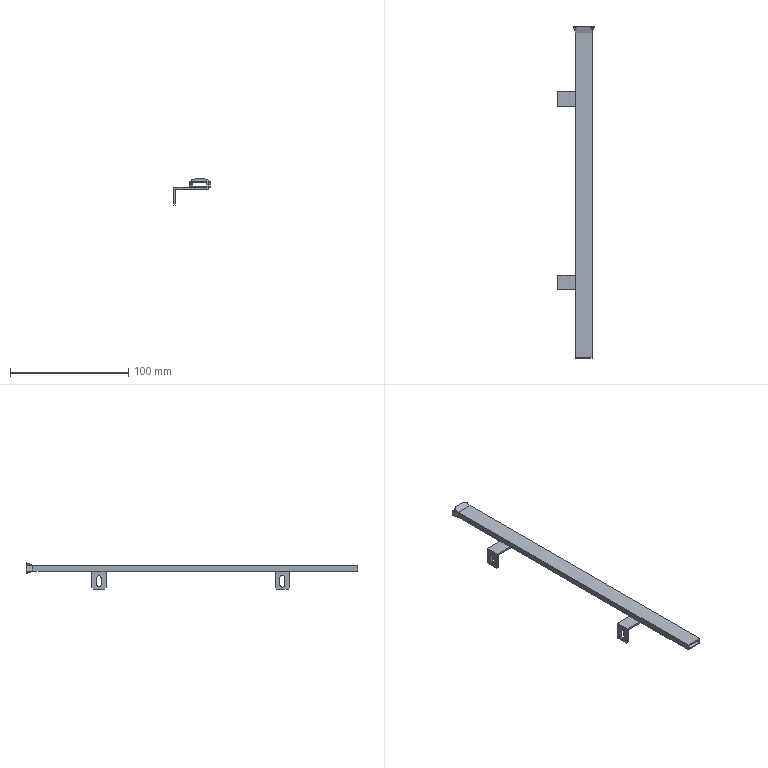Part | SolidWorks | features ICE 5, Fillet 3, Chamfer 1, Extrusion 1, LPattern 1, MirrorPattern 1 | 1 solid | 63 faces | box 30.899 x 280.673 x 21.992 mm | volume 10987 mm3 | plane 49 | cylinder 14 | commonest cylinder face diameters 4 x5 2 x4 3.5 x3 6 x2